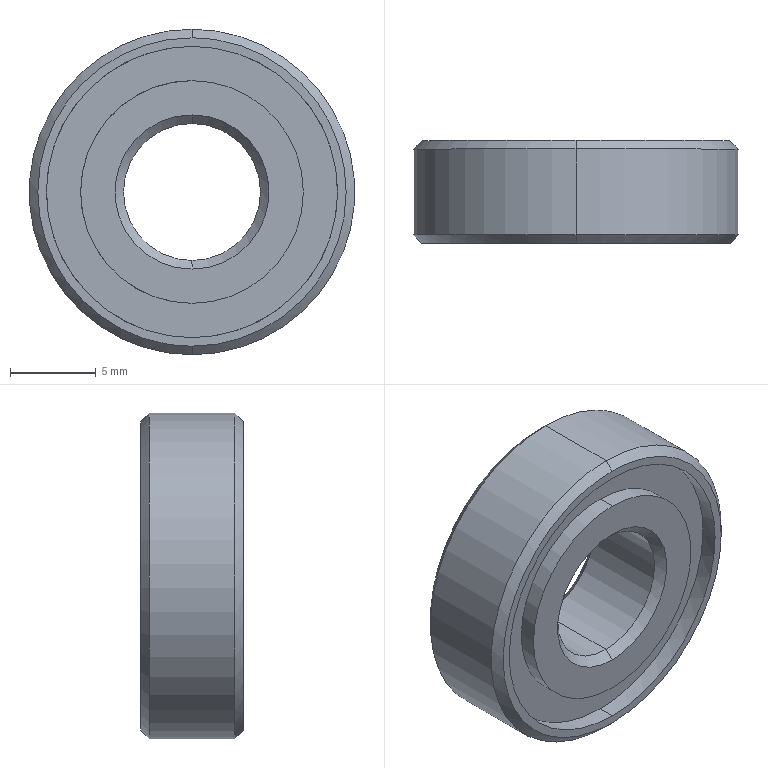Part | STEP file | PN_0010_Default<As Machined> | 1 solid | 26 faces | box 19 x 6 x 19 mm | volume 1190 mm3 | cylinder 12 | cone 8 | plane 6 | commonest cylinder face diameters 13 x4 17 x4 8 x2 19 x2
STEP:
#1=CARTESIAN_POINT('',(0.,1.,6.5));
#2=VERTEX_POINT('',#1);
#3=CARTESIAN_POINT('',(0.,1.,-6.5));
#4=VERTEX_POINT('',#3);
#5=CARTESIAN_POINT('',(0.,1.,0.));
#6=DIRECTION('',(0.,-1.,0.));
#7=AXIS2_PLACEMENT_3D('',#5,#6,$);
#8=CIRCLE('',#7,6.5);
#9=EDGE_CURVE('',#2,#4,#8,.F.);
#10=ORIENTED_EDGE('',*,*,#9,.F.);
#11=CARTESIAN_POINT('',(0.,0.,6.5));
#12=VERTEX_POINT('',#11);
#13=CARTESIAN_POINT('',(0.,1.,6.5));
#14=DIRECTION('',(0.,-1.,0.));
#15=VECTOR('',#14,1.);
#16=LINE('',#13,#15);
#17=EDGE_CURVE('',#2,#12,#16,.T.);
#18=ORIENTED_EDGE('',*,*,#17,.T.);
#19=CARTESIAN_POINT('',(0.,0.,-6.5));
#20=VERTEX_POINT('',#19);
#21=CARTESIAN_POINT('',(0.,0.,0.));
#22=DIRECTION('',(0.,-1.,0.));
#23=AXIS2_PLACEMENT_3D('',#21,#22,$);
#24=CIRCLE('',#23,6.5);
#25=EDGE_CURVE('',#12,#20,#24,.F.);
#26=ORIENTED_EDGE('',*,*,#25,.T.);
#27=CARTESIAN_POINT('',(0.,1.,-6.5));
#28=DIRECTION('',(0.,-1.,0.));
#29=VECTOR('',#28,1.);
#30=LINE('',#27,#29);
#31=EDGE_CURVE('',#4,#20,#30,.T.);
#32=ORIENTED_EDGE('',*,*,#31,.F.);
#33=EDGE_LOOP('',(#10,#18,#26,#32));
#34=FACE_OUTER_BOUND('',#33,.T.);
#35=CARTESIAN_POINT('',(0.,1.,0.));
#36=DIRECTION('',(0.,-1.,0.));
#37=DIRECTION('',(0.,0.,-1.));
#38=AXIS2_PLACEMENT_3D('',#35,#36,#37);
#39=CYLINDRICAL_SURFACE('',#38,6.5);
#40=ADVANCED_FACE('',(#34),#39,.T.);
#41=CARTESIAN_POINT('',(0.,1.,-8.5));
#42=VERTEX_POINT('',#41);
#43=CARTESIAN_POINT('',(0.,1.,8.5));
#44=VERTEX_POINT('',#43);
#45=CARTESIAN_POINT('',(0.,1.,-8.5));
#46=CARTESIAN_POINT('',(-0.857,1.,-8.5));
#47=CARTESIAN_POINT('',(-1.714,1.,-8.392));
#48=CARTESIAN_POINT('',(-2.553,1.,-8.176));
#49=CARTESIAN_POINT('',(-4.158,1.,-7.537));
#50=CARTESIAN_POINT('',(-5.554,1.,-6.52));
#51=CARTESIAN_POINT('',(-6.184,1.,-5.926));
#52=CARTESIAN_POINT('',(-7.281,1.,-4.591));
#53=CARTESIAN_POINT('',(-8.013,1.,-3.026));
#54=CARTESIAN_POINT('',(-8.277,1.,-2.202));
#55=CARTESIAN_POINT('',(-8.593,1.,-0.5032));
#56=CARTESIAN_POINT('',(-8.478,1.,1.22));
#57=CARTESIAN_POINT('',(-8.311,1.,2.07));
#58=CARTESIAN_POINT('',(-7.767,1.,3.71));
#59=CARTESIAN_POINT('',(-6.834,1.,5.164));
#60=CARTESIAN_POINT('',(-6.277,1.,5.827));
#61=CARTESIAN_POINT('',(-5.009,1.,7.));
#62=CARTESIAN_POINT('',(-3.49,1.,7.822));
#63=CARTESIAN_POINT('',(-2.682,1.,8.135));
#64=CARTESIAN_POINT('',(-1.649,1.,8.39));
#65=CARTESIAN_POINT('',(-0.5965,1.,8.483));
#66=CARTESIAN_POINT('',(-0.3976,1.,8.494));
#67=CARTESIAN_POINT('',(-0.1988,1.,8.5));
#68=CARTESIAN_POINT('',(0.,1.,8.5));
#69=B_SPLINE_CURVE_WITH_KNOTS('',5,(#45,#46,#47,#48,#49,#50,#51,#52,#53,#54,#55,#56,#57,#58,#59,#60,#61,#62,#63,#64,#65,#66,#67,#68),.UNSPECIFIED.,.F.,.U.,(6,3,3,3,3,3,3,6),(0.,6.06,12.119,18.179,24.239,30.298,36.358,37.764),.UNSPECIFIED.);
#70=EDGE_CURVE('',#42,#44,#69,.T.);
#71=ORIENTED_EDGE('',*,*,#70,.F.);
#72=CARTESIAN_POINT('',(0.,1.,8.5));
#73=CARTESIAN_POINT('',(0.857,1.,8.5));
#74=CARTESIAN_POINT('',(1.714,1.,8.392));
#75=CARTESIAN_POINT('',(2.553,1.,8.176));
#76=CARTESIAN_POINT('',(4.158,1.,7.537));
#77=CARTESIAN_POINT('',(5.554,1.,6.52));
#78=CARTESIAN_POINT('',(6.184,1.,5.926));
#79=CARTESIAN_POINT('',(7.281,1.,4.591));
#80=CARTESIAN_POINT('',(8.013,1.,3.026));
#81=CARTESIAN_POINT('',(8.277,1.,2.202));
#82=CARTESIAN_POINT('',(8.593,1.,0.5032));
#83=CARTESIAN_POINT('',(8.478,1.,-1.22));
#84=CARTESIAN_POINT('',(8.311,1.,-2.07));
#85=CARTESIAN_POINT('',(7.767,1.,-3.71));
#86=CARTESIAN_POINT('',(6.834,1.,-5.164));
#87=CARTESIAN_POINT('',(6.277,1.,-5.827));
#88=CARTESIAN_POINT('',(5.009,1.,-7.));
#89=CARTESIAN_POINT('',(3.49,1.,-7.822));
#90=CARTESIAN_POINT('',(2.682,1.,-8.135));
#91=CARTESIAN_POINT('',(1.649,1.,-8.39));
#92=CARTESIAN_POINT('',(0.5965,1.,-8.483));
#93=CARTESIAN_POINT('',(0.3976,1.,-8.494));
#94=CARTESIAN_POINT('',(0.1988,1.,-8.5));
#95=CARTESIAN_POINT('',(0.,1.,-8.5));
#96=B_SPLINE_CURVE_WITH_KNOTS('',5,(#72,#73,#74,#75,#76,#77,#78,#79,#80,#81,#82,#83,#84,#85,#86,#87,#88,#89,#90,#91,#92,#93,#94,#95),.UNSPECIFIED.,.F.,.U.,(6,3,3,3,3,3,3,6),(0.,6.06,12.119,18.179,24.239,30.298,36.358,37.764),.UNSPECIFIED.);
#97=EDGE_CURVE('',#44,#42,#96,.T.);
#98=ORIENTED_EDGE('',*,*,#97,.F.);
#99=EDGE_LOOP('',(#71,#98));
#100=FACE_OUTER_BOUND('',#99,.T.);
#101=CARTESIAN_POINT('',(0.,1.,-6.5));
#102=CARTESIAN_POINT('',(-0.6245,1.,-6.5));
#103=CARTESIAN_POINT('',(-1.249,1.,-6.425));
#104=CARTESIAN_POINT('',(-1.861,1.,-6.275));
#105=CARTESIAN_POINT('',(-3.038,1.,-5.831));
#106=CARTESIAN_POINT('',(-4.077,1.,-5.121));
#107=CARTESIAN_POINT('',(-4.551,1.,-4.705));
#108=CARTESIAN_POINT('',(-5.389,1.,-3.767));
#109=CARTESIAN_POINT('',(-5.982,1.,-2.657));
#110=CARTESIAN_POINT('',(-6.21,1.,-2.069));
#111=CARTESIAN_POINT('',(-6.52,1.,-0.85));
#112=CARTESIAN_POINT('',(-6.533,1.,0.4079));
#113=CARTESIAN_POINT('',(-6.463,1.,1.035));
#114=CARTESIAN_POINT('',(-6.175,1.,2.259));
#115=CARTESIAN_POINT('',(-5.605,1.,3.381));
#116=CARTESIAN_POINT('',(-5.253,1.,3.904));
#117=CARTESIAN_POINT('',(-4.432,1.,4.857));
#118=CARTESIAN_POINT('',(-3.408,1.,5.588));
#119=CARTESIAN_POINT('',(-2.855,1.,5.89));
#120=CARTESIAN_POINT('',(-1.955,1.,6.248));
#121=CARTESIAN_POINT('',(-1.009,1.,6.434));
#122=CARTESIAN_POINT('',(-0.6741,1.,6.478));
#123=CARTESIAN_POINT('',(-0.3371,1.,6.5));
#124=CARTESIAN_POINT('',(0.,1.,6.5));
#125=B_SPLINE_CURVE_WITH_KNOTS('',5,(#101,#102,#103,#104,#105,#106,#107,#108,#109,#110,#111,#112,#113,#114,#115,#116,#117,#118,#119,#120,#121,#122,#123,#124),.UNSPECIFIED.,.F.,.U.,(6,3,3,3,3,3,3,6),(0.,4.416,8.832,13.248,17.663,22.079,26.495,28.878),.UNSPECIFIED.);
#126=EDGE_CURVE('',#4,#2,#125,.T.);
#127=ORIENTED_EDGE('',*,*,#126,.T.);
#128=ORIENTED_EDGE('',*,*,#9,.T.);
#129=EDGE_LOOP('',(#127,#128));
#130=FACE_BOUND('',#129,.T.);
#131=CARTESIAN_POINT('',(0.,1.,0.));
#132=DIRECTION('',(0.,-1.,0.));
#133=DIRECTION('',(0.,0.,1.));
#134=AXIS2_PLACEMENT_3D('',#131,#132,#133);
#135=PLANE('',#134);
#136=ADVANCED_FACE('',(#100,#130),#135,.T.);
#137=ORIENTED_EDGE('',*,*,#17,.F.);
#138=ORIENTED_EDGE('',*,*,#126,.F.);
#139=ORIENTED_EDGE('',*,*,#31,.T.);
#140=CARTESIAN_POINT('',(0.,0.,0.));
#141=DIRECTION('',(0.,-1.,0.));
#142=AXIS2_PLACEMENT_3D('',#140,#141,$);
#143=CIRCLE('',#142,6.5);
#144=EDGE_CURVE('',#20,#12,#143,.F.);
#145=ORIENTED_EDGE('',*,*,#144,.T.);
#146=EDGE_LOOP('',(#137,#138,#139,#145));
#147=FACE_OUTER_BOUND('',#146,.T.);
#148=CARTESIAN_POINT('',(0.,1.,0.));
#149=DIRECTION('',(0.,-1.,0.));
#150=DIRECTION('',(0.,0.,1.));
#151=AXIS2_PLACEMENT_3D('',#148,#149,#150);
#152=CYLINDRICAL_SURFACE('',#151,6.5);
#153=ADVANCED_FACE('',(#147),#152,.T.);
#154=ORIENTED_EDGE('',*,*,#144,.F.);
#155=ORIENTED_EDGE('',*,*,#25,.F.);
#156=EDGE_LOOP('',(#154,#155));
#157=FACE_OUTER_BOUND('',#156,.T.);
#158=CARTESIAN_POINT('',(0.,0.,-4.5));
#159=VERTEX_POINT('',#158);
#160=CARTESIAN_POINT('',(0.,0.,4.5));
#161=VERTEX_POINT('',#160);
#162=CARTESIAN_POINT('',(0.,0.,0.));
#163=DIRECTION('',(0.,1.,0.));
#164=AXIS2_PLACEMENT_3D('',#162,#163,$);
#165=CIRCLE('',#164,4.5);
#166=EDGE_CURVE('',#159,#161,#165,.T.);
#167=ORIENTED_EDGE('',*,*,#166,.T.);
#168=CARTESIAN_POINT('',(0.,0.,0.));
#169=DIRECTION('',(0.,1.,0.));
#170=AXIS2_PLACEMENT_3D('',#168,#169,$);
#171=CIRCLE('',#170,4.5);
#172=EDGE_CURVE('',#161,#159,#171,.T.);
#173=ORIENTED_EDGE('',*,*,#172,.T.);
#174=EDGE_LOOP('',(#167,#173));
#175=FACE_BOUND('',#174,.T.);
#176=CARTESIAN_POINT('',(0.,0.,0.));
#177=DIRECTION('',(0.,1.,0.));
#178=DIRECTION('',(0.,0.,1.));
#179=AXIS2_PLACEMENT_3D('',#176,#177,#178);
#180=PLANE('',#179);
#181=ADVANCED_FACE('',(#157,#175),#180,.F.);
#182=ORIENTED_EDGE('',*,*,#70,.T.);
#183=CARTESIAN_POINT('',(0.,0.,8.5));
#184=VERTEX_POINT('',#183);
#185=CARTESIAN_POINT('',(0.,1.,8.5));
#186=DIRECTION('',(0.,-1.,0.));
#187=VECTOR('',#186,1.);
#188=LINE('',#185,#187);
#189=EDGE_CURVE('',#44,#184,#188,.T.);
#190=ORIENTED_EDGE('',*,*,#189,.T.);
#191=CARTESIAN_POINT('',(0.,0.,-8.5));
#192=VERTEX_POINT('',#191);
#193=CARTESIAN_POINT('',(0.,0.,0.));
#194=DIRECTION('',(0.,-1.,0.));
#195=AXIS2_PLACEMENT_3D('',#193,#194,$);
#196=CIRCLE('',#195,8.5);
#197=EDGE_CURVE('',#192,#184,#196,.F.);
#198=ORIENTED_EDGE('',*,*,#197,.F.);
#199=CARTESIAN_POINT('',(0.,1.,-8.5));
#200=DIRECTION('',(0.,-1.,0.));
#201=VECTOR('',#200,1.);
#202=LINE('',#199,#201);
#203=EDGE_CURVE('',#42,#192,#202,.T.);
#204=ORIENTED_EDGE('',*,*,#203,.F.);
#205=EDGE_LOOP('',(#182,#190,#198,#204));
#206=FACE_OUTER_BOUND('',#205,.T.);
#207=CARTESIAN_POINT('',(0.,1.,0.));
#208=DIRECTION('',(0.,-1.,0.));
#209=DIRECTION('',(0.,0.,1.));
#210=AXIS2_PLACEMENT_3D('',#207,#208,#209);
#211=CYLINDRICAL_SURFACE('',#210,8.5);
#212=ADVANCED_FACE('',(#206),#211,.F.);
#213=ORIENTED_EDGE('',*,*,#189,.F.);
#214=ORIENTED_EDGE('',*,*,#97,.T.);
#215=ORIENTED_EDGE('',*,*,#203,.T.);
#216=CARTESIAN_POINT('',(0.,0.,0.));
#217=DIRECTION('',(0.,-1.,0.));
#218=AXIS2_PLACEMENT_3D('',#216,#217,$);
#219=CIRCLE('',#218,8.5);
#220=EDGE_CURVE('',#184,#192,#219,.F.);
#221=ORIENTED_EDGE('',*,*,#220,.F.);
#222=EDGE_LOOP('',(#213,#214,#215,#221));
#223=FACE_OUTER_BOUND('',#222,.T.);
#224=CARTESIAN_POINT('',(0.,1.,0.));
#225=DIRECTION('',(0.,-1.,0.));
#226=DIRECTION('',(0.,0.,-1.));
#227=AXIS2_PLACEMENT_3D('',#224,#225,#226);
#228=CYLINDRICAL_SURFACE('',#227,8.5);
#229=ADVANCED_FACE('',(#223),#228,.F.);
#230=CARTESIAN_POINT('',(0.,0.5,4.));
#231=VERTEX_POINT('',#230);
#232=CARTESIAN_POINT('',(0.,0.5,-4.));
#233=VERTEX_POINT('',#232);
#234=CARTESIAN_POINT('',(0.,0.5,0.));
#235=DIRECTION('',(0.,-1.,0.));
#236=AXIS2_PLACEMENT_3D('',#234,#235,$);
#237=CIRCLE('',#236,4.);
#238=EDGE_CURVE('',#231,#233,#237,.T.);
#239=ORIENTED_EDGE('',*,*,#238,.F.);
#240=CARTESIAN_POINT('',(0.,-353551.141,353555.641));
#241=DIRECTION('',(0.,-0.7071,0.7071));
#242=VECTOR('',#241,1.);
#243=LINE('',#240,#242);
#244=EDGE_CURVE('',#231,#161,#243,.T.);
#245=ORIENTED_EDGE('',*,*,#244,.T.);
#246=ORIENTED_EDGE('',*,*,#166,.F.);
#247=CARTESIAN_POINT('',(0.,-353551.141,-353555.641));
#248=DIRECTION('',(0.,-0.7071,-0.7071));
#249=VECTOR('',#248,1.);
#250=LINE('',#247,#249);
#251=EDGE_CURVE('',#233,#159,#250,.T.);
#252=ORIENTED_EDGE('',*,*,#251,.F.);
#253=EDGE_LOOP('',(#239,#245,#246,#252));
#254=FACE_OUTER_BOUND('',#253,.T.);
#255=CARTESIAN_POINT('',(0.,0.,0.));
#256=DIRECTION('',(0.,-1.,0.));
#257=DIRECTION('',(0.,0.,1.));
#258=AXIS2_PLACEMENT_3D('',#255,#256,#257);
#259=CONICAL_SURFACE('',#258,4.5,0.7854);
#260=ADVANCED_FACE('',(#254),#259,.F.);
#261=ORIENTED_EDGE('',*,*,#244,.F.);
#262=CARTESIAN_POINT('',(0.,0.5,0.));
#263=DIRECTION('',(0.,-1.,0.));
#264=AXIS2_PLACEMENT_3D('',#262,#263,$);
#265=CIRCLE('',#264,4.);
#266=EDGE_CURVE('',#233,#231,#265,.T.);
#267=ORIENTED_EDGE('',*,*,#266,.F.);
#268=ORIENTED_EDGE('',*,*,#251,.T.);
#269=ORIENTED_EDGE('',*,*,#172,.F.);
#270=EDGE_LOOP('',(#261,#267,#268,#269));
#271=FACE_OUTER_BOUND('',#270,.T.);
#272=CARTESIAN_POINT('',(0.,0.,0.));
#273=DIRECTION('',(0.,-1.,0.));
#274=DIRECTION('',(0.,0.,-1.));
#275=AXIS2_PLACEMENT_3D('',#272,#273,#274);
#276=CONICAL_SURFACE('',#275,4.5,0.7854);
#277=ADVANCED_FACE('',(#271),#276,.F.);
#278=CARTESIAN_POINT('',(0.,0.,9.));
#279=VERTEX_POINT('',#278);
#280=CARTESIAN_POINT('',(0.,0.,-9.));
#281=VERTEX_POINT('',#280);
#282=CARTESIAN_POINT('',(0.,0.,9.));
#283=CARTESIAN_POINT('',(-0.8818,0.,9.));
#284=CARTESIAN_POINT('',(-1.764,0.,8.892));
#285=CARTESIAN_POINT('',(-2.628,0.,8.676));
#286=CARTESIAN_POINT('',(-4.286,0.,8.037));
#287=CARTESIAN_POINT('',(-5.74,0.,7.016));
#288=CARTESIAN_POINT('',(-6.401,0.,6.419));
#289=CARTESIAN_POINT('',(-7.563,0.,5.075));
#290=CARTESIAN_POINT('',(-8.366,0.,3.49));
#291=CARTESIAN_POINT('',(-8.669,0.,2.652));
#292=CARTESIAN_POINT('',(-9.061,0.,0.9193));
#293=CARTESIAN_POINT('',(-9.025,0.,-0.8571));
#294=CARTESIAN_POINT('',(-8.897,0.,-1.739));
#295=CARTESIAN_POINT('',(-8.428,0.,-3.453));
#296=CARTESIAN_POINT('',(-7.56,0.,-5.003));
#297=CARTESIAN_POINT('',(-7.032,0.,-5.721));
#298=CARTESIAN_POINT('',(-5.812,0.,-7.012));
#299=CARTESIAN_POINT('',(-4.317,0.,-7.971));
#300=CARTESIAN_POINT('',(-3.513,0.,-8.357));
#301=CARTESIAN_POINT('',(-2.324,0.,-8.756));
#302=CARTESIAN_POINT('',(-1.091,0.,-8.945));
#303=CARTESIAN_POINT('',(-0.7273,0.,-8.982));
#304=CARTESIAN_POINT('',(-0.3637,0.,-9.));
#305=CARTESIAN_POINT('',(0.,0.,-9.));
#306=B_SPLINE_CURVE_WITH_KNOTS('',5,(#282,#283,#284,#285,#286,#287,#288,#289,#290,#291,#292,#293,#294,#295,#296,#297,#298,#299,#300,#301,#302,#303,#304,#305),.UNSPECIFIED.,.F.,.U.,(6,3,3,3,3,3,3,6),(0.,6.235,12.471,18.706,24.941,31.177,37.412,39.983),.UNSPECIFIED.);
#307=EDGE_CURVE('',#279,#281,#306,.T.);
#308=ORIENTED_EDGE('',*,*,#307,.T.);
#309=CARTESIAN_POINT('',(0.,0.,-9.));
#310=CARTESIAN_POINT('',(0.8818,0.,-9.));
#311=CARTESIAN_POINT('',(1.764,0.,-8.892));
#312=CARTESIAN_POINT('',(2.628,0.,-8.676));
#313=CARTESIAN_POINT('',(4.286,0.,-8.037));
#314=CARTESIAN_POINT('',(5.74,0.,-7.016));
#315=CARTESIAN_POINT('',(6.401,0.,-6.419));
#316=CARTESIAN_POINT('',(7.563,0.,-5.075));
#317=CARTESIAN_POINT('',(8.366,0.,-3.49));
#318=CARTESIAN_POINT('',(8.669,0.,-2.652));
#319=CARTESIAN_POINT('',(9.061,0.,-0.9193));
#320=CARTESIAN_POINT('',(9.025,0.,0.8571));
#321=CARTESIAN_POINT('',(8.897,0.,1.739));
#322=CARTESIAN_POINT('',(8.428,0.,3.453));
#323=CARTESIAN_POINT('',(7.56,0.,5.003));
#324=CARTESIAN_POINT('',(7.032,0.,5.721));
#325=CARTESIAN_POINT('',(5.812,0.,7.012));
#326=CARTESIAN_POINT('',(4.317,0.,7.971));
#327=CARTESIAN_POINT('',(3.513,0.,8.357));
#328=CARTESIAN_POINT('',(2.324,0.,8.756));
#329=CARTESIAN_POINT('',(1.091,0.,8.945));
#330=CARTESIAN_POINT('',(0.7273,0.,8.982));
#331=CARTESIAN_POINT('',(0.3637,0.,9.));
#332=CARTESIAN_POINT('',(0.,0.,9.));
#333=B_SPLINE_CURVE_WITH_KNOTS('',5,(#309,#310,#311,#312,#313,#314,#315,#316,#317,#318,#319,#320,#321,#322,#323,#324,#325,#326,#327,#328,#329,#330,#331,#332),.UNSPECIFIED.,.F.,.U.,(6,3,3,3,3,3,3,6),(0.,6.235,12.471,18.706,24.941,31.177,37.412,39.983),.UNSPECIFIED.);
#334=EDGE_CURVE('',#281,#279,#333,.T.);
#335=ORIENTED_EDGE('',*,*,#334,.T.);
#336=EDGE_LOOP('',(#308,#335));
#337=FACE_OUTER_BOUND('',#336,.T.);
#338=ORIENTED_EDGE('',*,*,#197,.T.);
#339=ORIENTED_EDGE('',*,*,#220,.T.);
#340=EDGE_LOOP('',(#338,#339));
#341=FACE_BOUND('',#340,.T.);
#342=CARTESIAN_POINT('',(0.,0.,0.));
#343=DIRECTION('',(0.,1.,0.));
#344=DIRECTION('',(0.,0.,1.));
#345=AXIS2_PLACEMENT_3D('',#342,#343,#344);
#346=PLANE('',#345);
#347=ADVANCED_FACE('',(#337,#341),#346,.F.);
#348=CARTESIAN_POINT('',(0.,5.5,-4.));
#349=VERTEX_POINT('',#348);
#350=CARTESIAN_POINT('',(0.,5.5,4.));
#351=VERTEX_POINT('',#350);
#352=CARTESIAN_POINT('',(0.,5.5,0.));
#353=DIRECTION('',(0.,-1.,0.));
#354=AXIS2_PLACEMENT_3D('',#352,#353,$);
#355=CIRCLE('',#354,4.);
#356=EDGE_CURVE('',#349,#351,#355,.F.);
#357=ORIENTED_EDGE('',*,*,#356,.T.);
#358=CARTESIAN_POINT('',(0.,6.,4.));
#359=DIRECTION('',(0.,-1.,0.));
#360=VECTOR('',#359,1.);
#361=LINE('',#358,#360);
#362=EDGE_CURVE('',#351,#231,#361,.T.);
#363=ORIENTED_EDGE('',*,*,#362,.T.);
#364=ORIENTED_EDGE('',*,*,#238,.T.);
#365=CARTESIAN_POINT('',(0.,6.,-4.));
#366=DIRECTION('',(0.,-1.,0.));
#367=VECTOR('',#366,1.);
#368=LINE('',#365,#367);
#369=EDGE_CURVE('',#349,#233,#368,.T.);
#370=ORIENTED_EDGE('',*,*,#369,.F.);
#371=EDGE_LOOP('',(#357,#363,#364,#370));
#372=FACE_OUTER_BOUND('',#371,.T.);
#373=CARTESIAN_POINT('',(0.,6.,0.));
#374=DIRECTION('',(0.,-1.,0.));
#375=DIRECTION('',(0.,0.,1.));
#376=AXIS2_PLACEMENT_3D('',#373,#374,#375);
#377=CYLINDRICAL_SURFACE('',#376,4.);
#378=ADVANCED_FACE('',(#372),#377,.F.);
#379=ORIENTED_EDGE('',*,*,#362,.F.);
#380=CARTESIAN_POINT('',(0.,5.5,0.));
#381=DIRECTION('',(0.,-1.,0.));
#382=AXIS2_PLACEMENT_3D('',#380,#381,$);
#383=CIRCLE('',#382,4.);
#384=EDGE_CURVE('',#351,#349,#383,.F.);
#385=ORIENTED_EDGE('',*,*,#384,.T.);
#386=ORIENTED_EDGE('',*,*,#369,.T.);
#387=ORIENTED_EDGE('',*,*,#266,.T.);
#388=EDGE_LOOP('',(#379,#385,#386,#387));
#389=FACE_OUTER_BOUND('',#388,.T.);
#390=CARTESIAN_POINT('',(0.,6.,0.));
#391=DIRECTION('',(0.,-1.,0.));
#392=DIRECTION('',(0.,0.,-1.));
#393=AXIS2_PLACEMENT_3D('',#390,#391,#392);
#394=CYLINDRICAL_SURFACE('',#393,4.);
#395=ADVANCED_FACE('',(#389),#394,.F.);
#396=CARTESIAN_POINT('',(0.,0.5,-9.5));
#397=VERTEX_POINT('',#396);
#398=CARTESIAN_POINT('',(0.,353549.141,-353558.141));
#399=DIRECTION('',(0.,0.7071,-0.7071));
#400=VECTOR('',#399,1.);
#401=LINE('',#398,#400);
#402=EDGE_CURVE('',#281,#397,#401,.T.);
#403=ORIENTED_EDGE('',*,*,#402,.F.);
#404=ORIENTED_EDGE('',*,*,#307,.F.);
#405=CARTESIAN_POINT('',(0.,0.5,9.5));
#406=VERTEX_POINT('',#405);
#407=CARTESIAN_POINT('',(0.,353549.141,353558.141));
#408=DIRECTION('',(0.,0.7071,0.7071));
#409=VECTOR('',#408,1.);
#410=LINE('',#407,#409);
#411=EDGE_CURVE('',#279,#406,#410,.T.);
#412=ORIENTED_EDGE('',*,*,#411,.T.);
#413=CARTESIAN_POINT('',(0.,0.5,0.));
#414=DIRECTION('',(0.,1.,0.));
#415=AXIS2_PLACEMENT_3D('',#413,#414,$);
#416=CIRCLE('',#415,9.5);
#417=EDGE_CURVE('',#397,#406,#416,.T.);
#418=ORIENTED_EDGE('',*,*,#417,.F.);
#419=EDGE_LOOP('',(#403,#404,#412,#418));
#420=FACE_OUTER_BOUND('',#419,.T.);
#421=CARTESIAN_POINT('',(0.,0.5,0.));
#422=DIRECTION('',(0.,1.,0.));
#423=DIRECTION('',(0.,0.,-1.));
#424=AXIS2_PLACEMENT_3D('',#421,#422,#423);
#425=CONICAL_SURFACE('',#424,9.5,0.7854);
#426=ADVANCED_FACE('',(#420),#425,.T.);
#427=ORIENTED_EDGE('',*,*,#334,.F.);
#428=ORIENTED_EDGE('',*,*,#402,.T.);
#429=CARTESIAN_POINT('',(0.,0.5,0.));
#430=DIRECTION('',(0.,1.,0.));
#431=AXIS2_PLACEMENT_3D('',#429,#430,$);
#432=CIRCLE('',#431,9.5);
#433=EDGE_CURVE('',#406,#397,#432,.T.);
#434=ORIENTED_EDGE('',*,*,#433,.F.);
#435=ORIENTED_EDGE('',*,*,#411,.F.);
#436=EDGE_LOOP('',(#427,#428,#434,#435));
#437=FACE_OUTER_BOUND('',#436,.T.);
#438=CARTESIAN_POINT('',(0.,0.5,0.));
#439=DIRECTION('',(0.,1.,0.));
#440=DIRECTION('',(0.,0.,1.));
#441=AXIS2_PLACEMENT_3D('',#438,#439,#440);
#442=CONICAL_SURFACE('',#441,9.5,0.7854);
#443=ADVANCED_FACE('',(#437),#442,.T.);
#444=ORIENTED_EDGE('',*,*,#356,.F.);
#445=CARTESIAN_POINT('',(0.,6.,-4.5));
#446=VERTEX_POINT('',#445);
#447=CARTESIAN_POINT('',(0.,353556.891,-353555.391));
#448=DIRECTION('',(0.,0.7071,-0.7071));
#449=VECTOR('',#448,1.);
#450=LINE('',#447,#449);
#451=EDGE_CURVE('',#349,#446,#450,.T.);
#452=ORIENTED_EDGE('',*,*,#451,.T.);
#453=CARTESIAN_POINT('',(0.,6.,4.5));
#454=VERTEX_POINT('',#453);
#455=CARTESIAN_POINT('',(0.,6.,0.));
#456=DIRECTION('',(0.,1.,0.));
#457=AXIS2_PLACEMENT_3D('',#455,#456,$);
#458=CIRCLE('',#457,4.5);
#459=EDGE_CURVE('',#454,#446,#458,.F.);
#460=ORIENTED_EDGE('',*,*,#459,.F.);
#461=CARTESIAN_POINT('',(0.,353556.891,353555.391));
#462=DIRECTION('',(0.,0.7071,0.7071));
#463=VECTOR('',#462,1.);
#464=LINE('',#461,#463);
#465=EDGE_CURVE('',#351,#454,#464,.T.);
#466=ORIENTED_EDGE('',*,*,#465,.F.);
#467=EDGE_LOOP('',(#444,#452,#460,#466));
#468=FACE_OUTER_BOUND('',#467,.T.);
#469=CARTESIAN_POINT('',(0.,5.5,0.));
#470=DIRECTION('',(0.,1.,0.));
#471=DIRECTION('',(0.,0.,-1.));
#472=AXIS2_PLACEMENT_3D('',#469,#470,#471);
#473=CONICAL_SURFACE('',#472,4.,0.7854);
#474=ADVANCED_FACE('',(#468),#473,.F.);
#475=ORIENTED_EDGE('',*,*,#451,.F.);
#476=ORIENTED_EDGE('',*,*,#384,.F.);
#477=ORIENTED_EDGE('',*,*,#465,.T.);
#478=CARTESIAN_POINT('',(0.,6.,0.));
#479=DIRECTION('',(0.,1.,0.));
#480=AXIS2_PLACEMENT_3D('',#478,#479,$);
#481=CIRCLE('',#480,4.5);
#482=EDGE_CURVE('',#446,#454,#481,.F.);
#483=ORIENTED_EDGE('',*,*,#482,.F.);
#484=EDGE_LOOP('',(#475,#476,#477,#483));
#485=FACE_OUTER_BOUND('',#484,.T.);
#486=CARTESIAN_POINT('',(0.,5.5,0.));
#487=DIRECTION('',(0.,1.,0.));
#488=DIRECTION('',(0.,0.,1.));
#489=AXIS2_PLACEMENT_3D('',#486,#487,#488);
#490=CONICAL_SURFACE('',#489,4.,0.7854);
#491=ADVANCED_FACE('',(#485),#490,.F.);
#492=CARTESIAN_POINT('',(0.,5.5,9.5));
#493=VERTEX_POINT('',#492);
#494=CARTESIAN_POINT('',(0.,6.,9.5));
#495=DIRECTION('',(0.,-1.,0.));
#496=VECTOR('',#495,1.);
#497=LINE('',#494,#496);
#498=EDGE_CURVE('',#493,#406,#497,.T.);
#499=ORIENTED_EDGE('',*,*,#498,.F.);
#500=CARTESIAN_POINT('',(0.,5.5,-9.5));
#501=VERTEX_POINT('',#500);
#502=CARTESIAN_POINT('',(0.,5.5,0.));
#503=DIRECTION('',(0.,-1.,0.));
#504=AXIS2_PLACEMENT_3D('',#502,#503,$);
#505=CIRCLE('',#504,9.5);
#506=EDGE_CURVE('',#493,#501,#505,.T.);
#507=ORIENTED_EDGE('',*,*,#506,.T.);
#508=CARTESIAN_POINT('',(0.,6.,-9.5));
#509=DIRECTION('',(0.,-1.,0.));
#510=VECTOR('',#509,1.);
#511=LINE('',#508,#510);
#512=EDGE_CURVE('',#501,#397,#511,.T.);
#513=ORIENTED_EDGE('',*,*,#512,.T.);
#514=ORIENTED_EDGE('',*,*,#417,.T.);
#515=EDGE_LOOP('',(#499,#507,#513,#514));
#516=FACE_OUTER_BOUND('',#515,.T.);
#517=CARTESIAN_POINT('',(0.,6.,0.));
#518=DIRECTION('',(0.,-1.,0.));
#519=DIRECTION('',(0.,0.,1.));
#520=AXIS2_PLACEMENT_3D('',#517,#518,#519);
#521=CYLINDRICAL_SURFACE('',#520,9.5);
#522=ADVANCED_FACE('',(#516),#521,.T.);
#523=CARTESIAN_POINT('',(0.,5.5,0.));
#524=DIRECTION('',(0.,-1.,0.));
#525=AXIS2_PLACEMENT_3D('',#523,#524,$);
#526=CIRCLE('',#525,9.5);
#527=EDGE_CURVE('',#501,#493,#526,.T.);
#528=ORIENTED_EDGE('',*,*,#527,.T.);
#529=ORIENTED_EDGE('',*,*,#498,.T.);
#530=ORIENTED_EDGE('',*,*,#433,.T.);
#531=ORIENTED_EDGE('',*,*,#512,.F.);
#532=EDGE_LOOP('',(#528,#529,#530,#531));
#533=FACE_OUTER_BOUND('',#532,.T.);
#534=CARTESIAN_POINT('',(0.,6.,0.));
#535=DIRECTION('',(0.,-1.,0.));
#536=DIRECTION('',(0.,0.,-1.));
#537=AXIS2_PLACEMENT_3D('',#534,#535,#536);
#538=CYLINDRICAL_SURFACE('',#537,9.5);
#539=ADVANCED_FACE('',(#533),#538,.T.);
#540=CARTESIAN_POINT('',(0.,6.,6.5));
#541=VERTEX_POINT('',#540);
#542=CARTESIAN_POINT('',(0.,6.,-6.5));
#543=VERTEX_POINT('',#542);
#544=CARTESIAN_POINT('',(0.,6.,0.));
#545=DIRECTION('',(0.,1.,0.));
#546=AXIS2_PLACEMENT_3D('',#544,#545,$);
#547=CIRCLE('',#546,6.5);
#548=EDGE_CURVE('',#541,#543,#547,.T.);
#549=ORIENTED_EDGE('',*,*,#548,.T.);
#550=CARTESIAN_POINT('',(0.,6.,0.));
#551=DIRECTION('',(0.,1.,0.));
#552=AXIS2_PLACEMENT_3D('',#550,#551,$);
#553=CIRCLE('',#552,6.5);
#554=EDGE_CURVE('',#543,#541,#553,.T.);
#555=ORIENTED_EDGE('',*,*,#554,.T.);
#556=EDGE_LOOP('',(#549,#555));
#557=FACE_OUTER_BOUND('',#556,.T.);
#558=ORIENTED_EDGE('',*,*,#459,.T.);
#559=ORIENTED_EDGE('',*,*,#482,.T.);
#560=EDGE_LOOP('',(#558,#559));
#561=FACE_BOUND('',#560,.T.);
#562=CARTESIAN_POINT('',(0.,6.,0.));
#563=DIRECTION('',(0.,1.,0.));
#564=DIRECTION('',(0.,0.,1.));
#565=AXIS2_PLACEMENT_3D('',#562,#563,#564);
#566=PLANE('',#565);
#567=ADVANCED_FACE('',(#557,#561),#566,.T.);
#568=CARTESIAN_POINT('',(0.,6.,9.));
#569=VERTEX_POINT('',#568);
#570=CARTESIAN_POINT('',(0.,-353542.891,353557.891));
#571=DIRECTION('',(0.,-0.7071,0.7071));
#572=VECTOR('',#571,1.);
#573=LINE('',#570,#572);
#574=EDGE_CURVE('',#569,#493,#573,.T.);
#575=ORIENTED_EDGE('',*,*,#574,.F.);
#576=CARTESIAN_POINT('',(0.,6.,-9.));
#577=VERTEX_POINT('',#576);
#578=CARTESIAN_POINT('',(0.,6.,0.));
#579=DIRECTION('',(0.,-1.,0.));
#580=AXIS2_PLACEMENT_3D('',#578,#579,$);
#581=CIRCLE('',#580,9.);
#582=EDGE_CURVE('',#577,#569,#581,.F.);
#583=ORIENTED_EDGE('',*,*,#582,.F.);
#584=CARTESIAN_POINT('',(0.,-353542.891,-353557.891));
#585=DIRECTION('',(0.,-0.7071,-0.7071));
#586=VECTOR('',#585,1.);
#587=LINE('',#584,#586);
#588=EDGE_CURVE('',#577,#501,#587,.T.);
#589=ORIENTED_EDGE('',*,*,#588,.T.);
#590=ORIENTED_EDGE('',*,*,#506,.F.);
#591=EDGE_LOOP('',(#575,#583,#589,#590));
#592=FACE_OUTER_BOUND('',#591,.T.);
#593=CARTESIAN_POINT('',(0.,6.,0.));
#594=DIRECTION('',(0.,-1.,0.));
#595=DIRECTION('',(0.,0.,1.));
#596=AXIS2_PLACEMENT_3D('',#593,#594,#595);
#597=CONICAL_SURFACE('',#596,9.,0.7854);
#598=ADVANCED_FACE('',(#592),#597,.T.);
#599=CARTESIAN_POINT('',(0.,6.,0.));
#600=DIRECTION('',(0.,-1.,0.));
#601=AXIS2_PLACEMENT_3D('',#599,#600,$);
#602=CIRCLE('',#601,9.);
#603=EDGE_CURVE('',#569,#577,#602,.F.);
#604=ORIENTED_EDGE('',*,*,#603,.F.);
#605=ORIENTED_EDGE('',*,*,#574,.T.);
#606=ORIENTED_EDGE('',*,*,#527,.F.);
#607=ORIENTED_EDGE('',*,*,#588,.F.);
#608=EDGE_LOOP('',(#604,#605,#606,#607));
#609=FACE_OUTER_BOUND('',#608,.T.);
#610=CARTESIAN_POINT('',(0.,6.,0.));
#611=DIRECTION('',(0.,-1.,0.));
#612=DIRECTION('',(0.,0.,-1.));
#613=AXIS2_PLACEMENT_3D('',#610,#611,#612);
#614=CONICAL_SURFACE('',#613,9.,0.7854);
#615=ADVANCED_FACE('',(#609),#614,.T.);
#616=CARTESIAN_POINT('',(0.,5.,6.5));
#617=VERTEX_POINT('',#616);
#618=CARTESIAN_POINT('',(0.,5.,-6.5));
#619=VERTEX_POINT('',#618);
#620=CARTESIAN_POINT('',(0.,5.,0.));
#621=DIRECTION('',(0.,1.,0.));
#622=AXIS2_PLACEMENT_3D('',#620,#621,$);
#623=CIRCLE('',#622,6.5);
#624=EDGE_CURVE('',#617,#619,#623,.T.);
#625=ORIENTED_EDGE('',*,*,#624,.T.);
#626=CARTESIAN_POINT('',(0.,5.,-6.5));
#627=DIRECTION('',(0.,1.,0.));
#628=VECTOR('',#627,1.);
#629=LINE('',#626,#628);
#630=EDGE_CURVE('',#619,#543,#629,.T.);
#631=ORIENTED_EDGE('',*,*,#630,.T.);
#632=ORIENTED_EDGE('',*,*,#548,.F.);
#633=CARTESIAN_POINT('',(0.,5.,6.5));
#634=DIRECTION('',(0.,1.,0.));
#635=VECTOR('',#634,1.);
#636=LINE('',#633,#635);
#637=EDGE_CURVE('',#617,#541,#636,.T.);
#638=ORIENTED_EDGE('',*,*,#637,.F.);
#639=EDGE_LOOP('',(#625,#631,#632,#638));
#640=FACE_OUTER_BOUND('',#639,.T.);
#641=CARTESIAN_POINT('',(0.,5.,0.));
#642=DIRECTION('',(0.,1.,0.));
#643=DIRECTION('',(0.,0.,1.));
#644=AXIS2_PLACEMENT_3D('',#641,#642,#643);
#645=CYLINDRICAL_SURFACE('',#644,6.5);
#646=ADVANCED_FACE('',(#640),#645,.T.);
#647=ORIENTED_EDGE('',*,*,#630,.F.);
#648=CARTESIAN_POINT('',(0.,5.,0.));
#649=DIRECTION('',(0.,1.,0.));
#650=AXIS2_PLACEMENT_3D('',#648,#649,$);
#651=CIRCLE('',#650,6.5);
#652=EDGE_CURVE('',#619,#617,#651,.T.);
#653=ORIENTED_EDGE('',*,*,#652,.T.);
#654=ORIENTED_EDGE('',*,*,#637,.T.);
#655=ORIENTED_EDGE('',*,*,#554,.F.);
#656=EDGE_LOOP('',(#647,#653,#654,#655));
#657=FACE_OUTER_BOUND('',#656,.T.);
#658=CARTESIAN_POINT('',(0.,5.,0.));
#659=DIRECTION('',(0.,1.,0.));
#660=DIRECTION('',(0.,0.,-1.));
#661=AXIS2_PLACEMENT_3D('',#658,#659,#660);
#662=CYLINDRICAL_SURFACE('',#661,6.5);
#663=ADVANCED_FACE('',(#657),#662,.T.);
#664=ORIENTED_EDGE('',*,*,#582,.T.);
#665=ORIENTED_EDGE('',*,*,#603,.T.);
#666=EDGE_LOOP('',(#664,#665));
#667=FACE_OUTER_BOUND('',#666,.T.);
#668=CARTESIAN_POINT('',(0.,6.,8.5));
#669=VERTEX_POINT('',#668);
#670=CARTESIAN_POINT('',(0.,6.,-8.5));
#671=VERTEX_POINT('',#670);
#672=CARTESIAN_POINT('',(0.,6.,0.));
#673=DIRECTION('',(0.,1.,0.));
#674=AXIS2_PLACEMENT_3D('',#672,#673,$);
#675=CIRCLE('',#674,8.5);
#676=EDGE_CURVE('',#669,#671,#675,.T.);
#677=ORIENTED_EDGE('',*,*,#676,.F.);
#678=CARTESIAN_POINT('',(0.,6.,0.));
#679=DIRECTION('',(0.,1.,0.));
#680=AXIS2_PLACEMENT_3D('',#678,#679,$);
#681=CIRCLE('',#680,8.5);
#682=EDGE_CURVE('',#671,#669,#681,.T.);
#683=ORIENTED_EDGE('',*,*,#682,.F.);
#684=EDGE_LOOP('',(#677,#683));
#685=FACE_BOUND('',#684,.T.);
#686=CARTESIAN_POINT('',(0.,6.,0.));
#687=DIRECTION('',(0.,1.,0.));
#688=DIRECTION('',(0.,0.,1.));
#689=AXIS2_PLACEMENT_3D('',#686,#687,#688);
#690=PLANE('',#689);
#691=ADVANCED_FACE('',(#667,#685),#690,.T.);
#692=CARTESIAN_POINT('',(0.,5.,8.5));
#693=VERTEX_POINT('',#692);
#694=CARTESIAN_POINT('',(0.,5.,-8.5));
#695=VERTEX_POINT('',#694);
#696=CARTESIAN_POINT('',(0.,5.,0.));
#697=DIRECTION('',(0.,1.,0.));
#698=AXIS2_PLACEMENT_3D('',#696,#697,$);
#699=CIRCLE('',#698,8.5);
#700=EDGE_CURVE('',#693,#695,#699,.T.);
#701=ORIENTED_EDGE('',*,*,#700,.T.);
#702=CARTESIAN_POINT('',(0.,5.,0.));
#703=DIRECTION('',(0.,1.,0.));
#704=AXIS2_PLACEMENT_3D('',#702,#703,$);
#705=CIRCLE('',#704,8.5);
#706=EDGE_CURVE('',#695,#693,#705,.T.);
#707=ORIENTED_EDGE('',*,*,#706,.T.);
#708=EDGE_LOOP('',(#701,#707));
#709=FACE_OUTER_BOUND('',#708,.T.);
#710=ORIENTED_EDGE('',*,*,#624,.F.);
#711=ORIENTED_EDGE('',*,*,#652,.F.);
#712=EDGE_LOOP('',(#710,#711));
#713=FACE_BOUND('',#712,.T.);
#714=CARTESIAN_POINT('',(0.,5.,0.));
#715=DIRECTION('',(0.,1.,0.));
#716=DIRECTION('',(0.,0.,1.));
#717=AXIS2_PLACEMENT_3D('',#714,#715,#716);
#718=PLANE('',#717);
#719=ADVANCED_FACE('',(#709,#713),#718,.T.);
#720=CARTESIAN_POINT('',(0.,5.,-8.5));
#721=DIRECTION('',(0.,1.,0.));
#722=VECTOR('',#721,1.);
#723=LINE('',#720,#722);
#724=EDGE_CURVE('',#695,#671,#723,.T.);
#725=ORIENTED_EDGE('',*,*,#724,.F.);
#726=ORIENTED_EDGE('',*,*,#700,.F.);
#727=CARTESIAN_POINT('',(0.,5.,8.5));
#728=DIRECTION('',(0.,1.,0.));
#729=VECTOR('',#728,1.);
#730=LINE('',#727,#729);
#731=EDGE_CURVE('',#693,#669,#730,.T.);
#732=ORIENTED_EDGE('',*,*,#731,.T.);
#733=ORIENTED_EDGE('',*,*,#676,.T.);
#734=EDGE_LOOP('',(#725,#726,#732,#733));
#735=FACE_OUTER_BOUND('',#734,.T.);
#736=CARTESIAN_POINT('',(0.,5.,0.));
#737=DIRECTION('',(0.,1.,0.));
#738=DIRECTION('',(0.,0.,1.));
#739=AXIS2_PLACEMENT_3D('',#736,#737,#738);
#740=CYLINDRICAL_SURFACE('',#739,8.5);
#741=ADVANCED_FACE('',(#735),#740,.F.);
#742=ORIENTED_EDGE('',*,*,#706,.F.);
#743=ORIENTED_EDGE('',*,*,#724,.T.);
#744=ORIENTED_EDGE('',*,*,#682,.T.);
#745=ORIENTED_EDGE('',*,*,#731,.F.);
#746=EDGE_LOOP('',(#742,#743,#744,#745));
#747=FACE_OUTER_BOUND('',#746,.T.);
#748=CARTESIAN_POINT('',(0.,5.,0.));
#749=DIRECTION('',(0.,1.,0.));
#750=DIRECTION('',(0.,0.,-1.));
#751=AXIS2_PLACEMENT_3D('',#748,#749,#750);
#752=CYLINDRICAL_SURFACE('',#751,8.5);
#753=ADVANCED_FACE('',(#747),#752,.F.);
#754=CLOSED_SHELL('',(#40,#136,#153,#181,#212,#229,#260,#277,#347,#378,#395,#426,#443,#474,#491,#522,#539,#567,#598,#615,#646,#663,#691,#719,#741,#753));
#755=MANIFOLD_SOLID_BREP('',#754);
#756=(LENGTH_UNIT()NAMED_UNIT(*)SI_UNIT(.MILLI.,.METRE.));
#757=UNCERTAINTY_MEASURE_WITH_UNIT(LENGTH_MEASURE(0.005),#756,'','');
#758=(NAMED_UNIT(*)PLANE_ANGLE_UNIT()SI_UNIT($,.RADIAN.));
#759=(NAMED_UNIT(*)SI_UNIT($,.STERADIAN.)SOLID_ANGLE_UNIT());
#760=(GEOMETRIC_REPRESENTATION_CONTEXT(3)GLOBAL_UNCERTAINTY_ASSIGNED_CONTEXT((#757))GLOBAL_UNIT_ASSIGNED_CONTEXT((#756,#758,#759))REPRESENTATION_CONTEXT('',''));
#761=ADVANCED_BREP_SHAPE_REPRESENTATION('',(#755),#760);